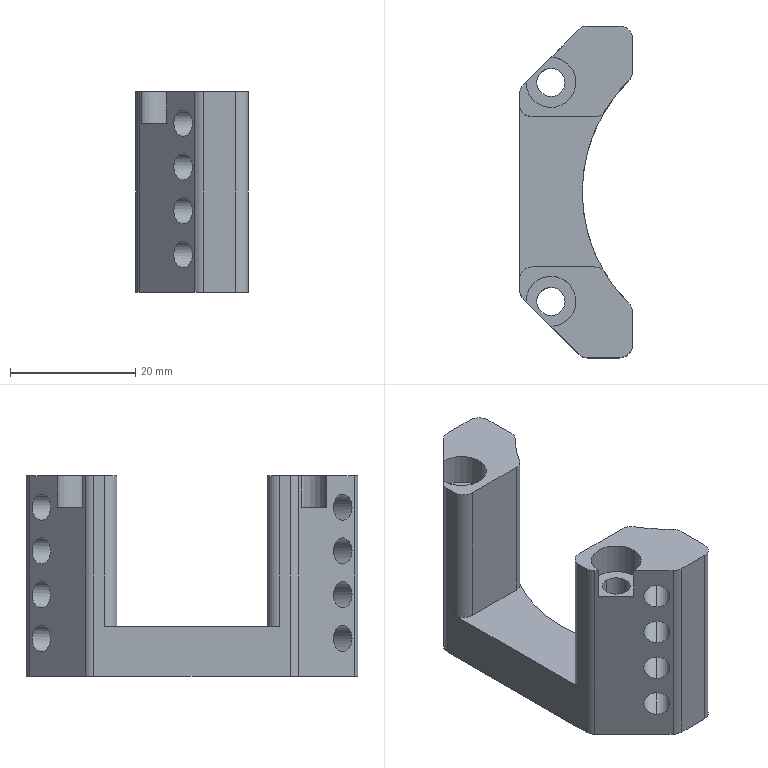NC program | Mastercam | posted with a generic post
Lines 1 to 41 of 15624:
%
O0000()
(MATERIAL - ALUMINUM MM - 2024)
( T24 | 100 FEM | H24 )
( T11 | 12 FEM | H11 )
( T4 | 4 FEM | H4 | XY STOCK TO LEAVE - .07 | Z STOCK TO LEAVE - .05 )
( T12 | 12 FEM | H12 | XY STOCK TO LEAVE - .2 | Z STOCK TO LEAVE - 0. )
( T5 | 4 CHM | H5 )
N100 G21
N110 G0 G17 G40 G49 G80 G90
N120 T24 M6
N130 G0 G90 G54 X-110. Y0. A0. S4000 M3
N140 G43 H24 Z52. M8
N150 Z4.
N160 G1 Z1.525 F600.
N170 X110. F3000.
N180 G0 Z51.525
N190 X-110.
N200 Z3.525
N210 G1 Z1.05 F600.
N220 X110. F3000.
N230 G0 Z51.05
N240 X-110.
N250 Z3.05
N260 G1 Z.575 F600.
N270 X110. F3000.
N280 G0 Z50.575
N290 X-110.
N300 Z2.575
N310 G1 Z.1 F600.
N320 X110. F3000.
N330 G0 Z50.1
N340 X-110.
N350 Z2.1
N360 G1 Z0. F600.
N370 X110. F1000.
N380 G0 Z50.
N390 M5
N400 G91 G28 Z0. M9
N410 A0.
N420 M01